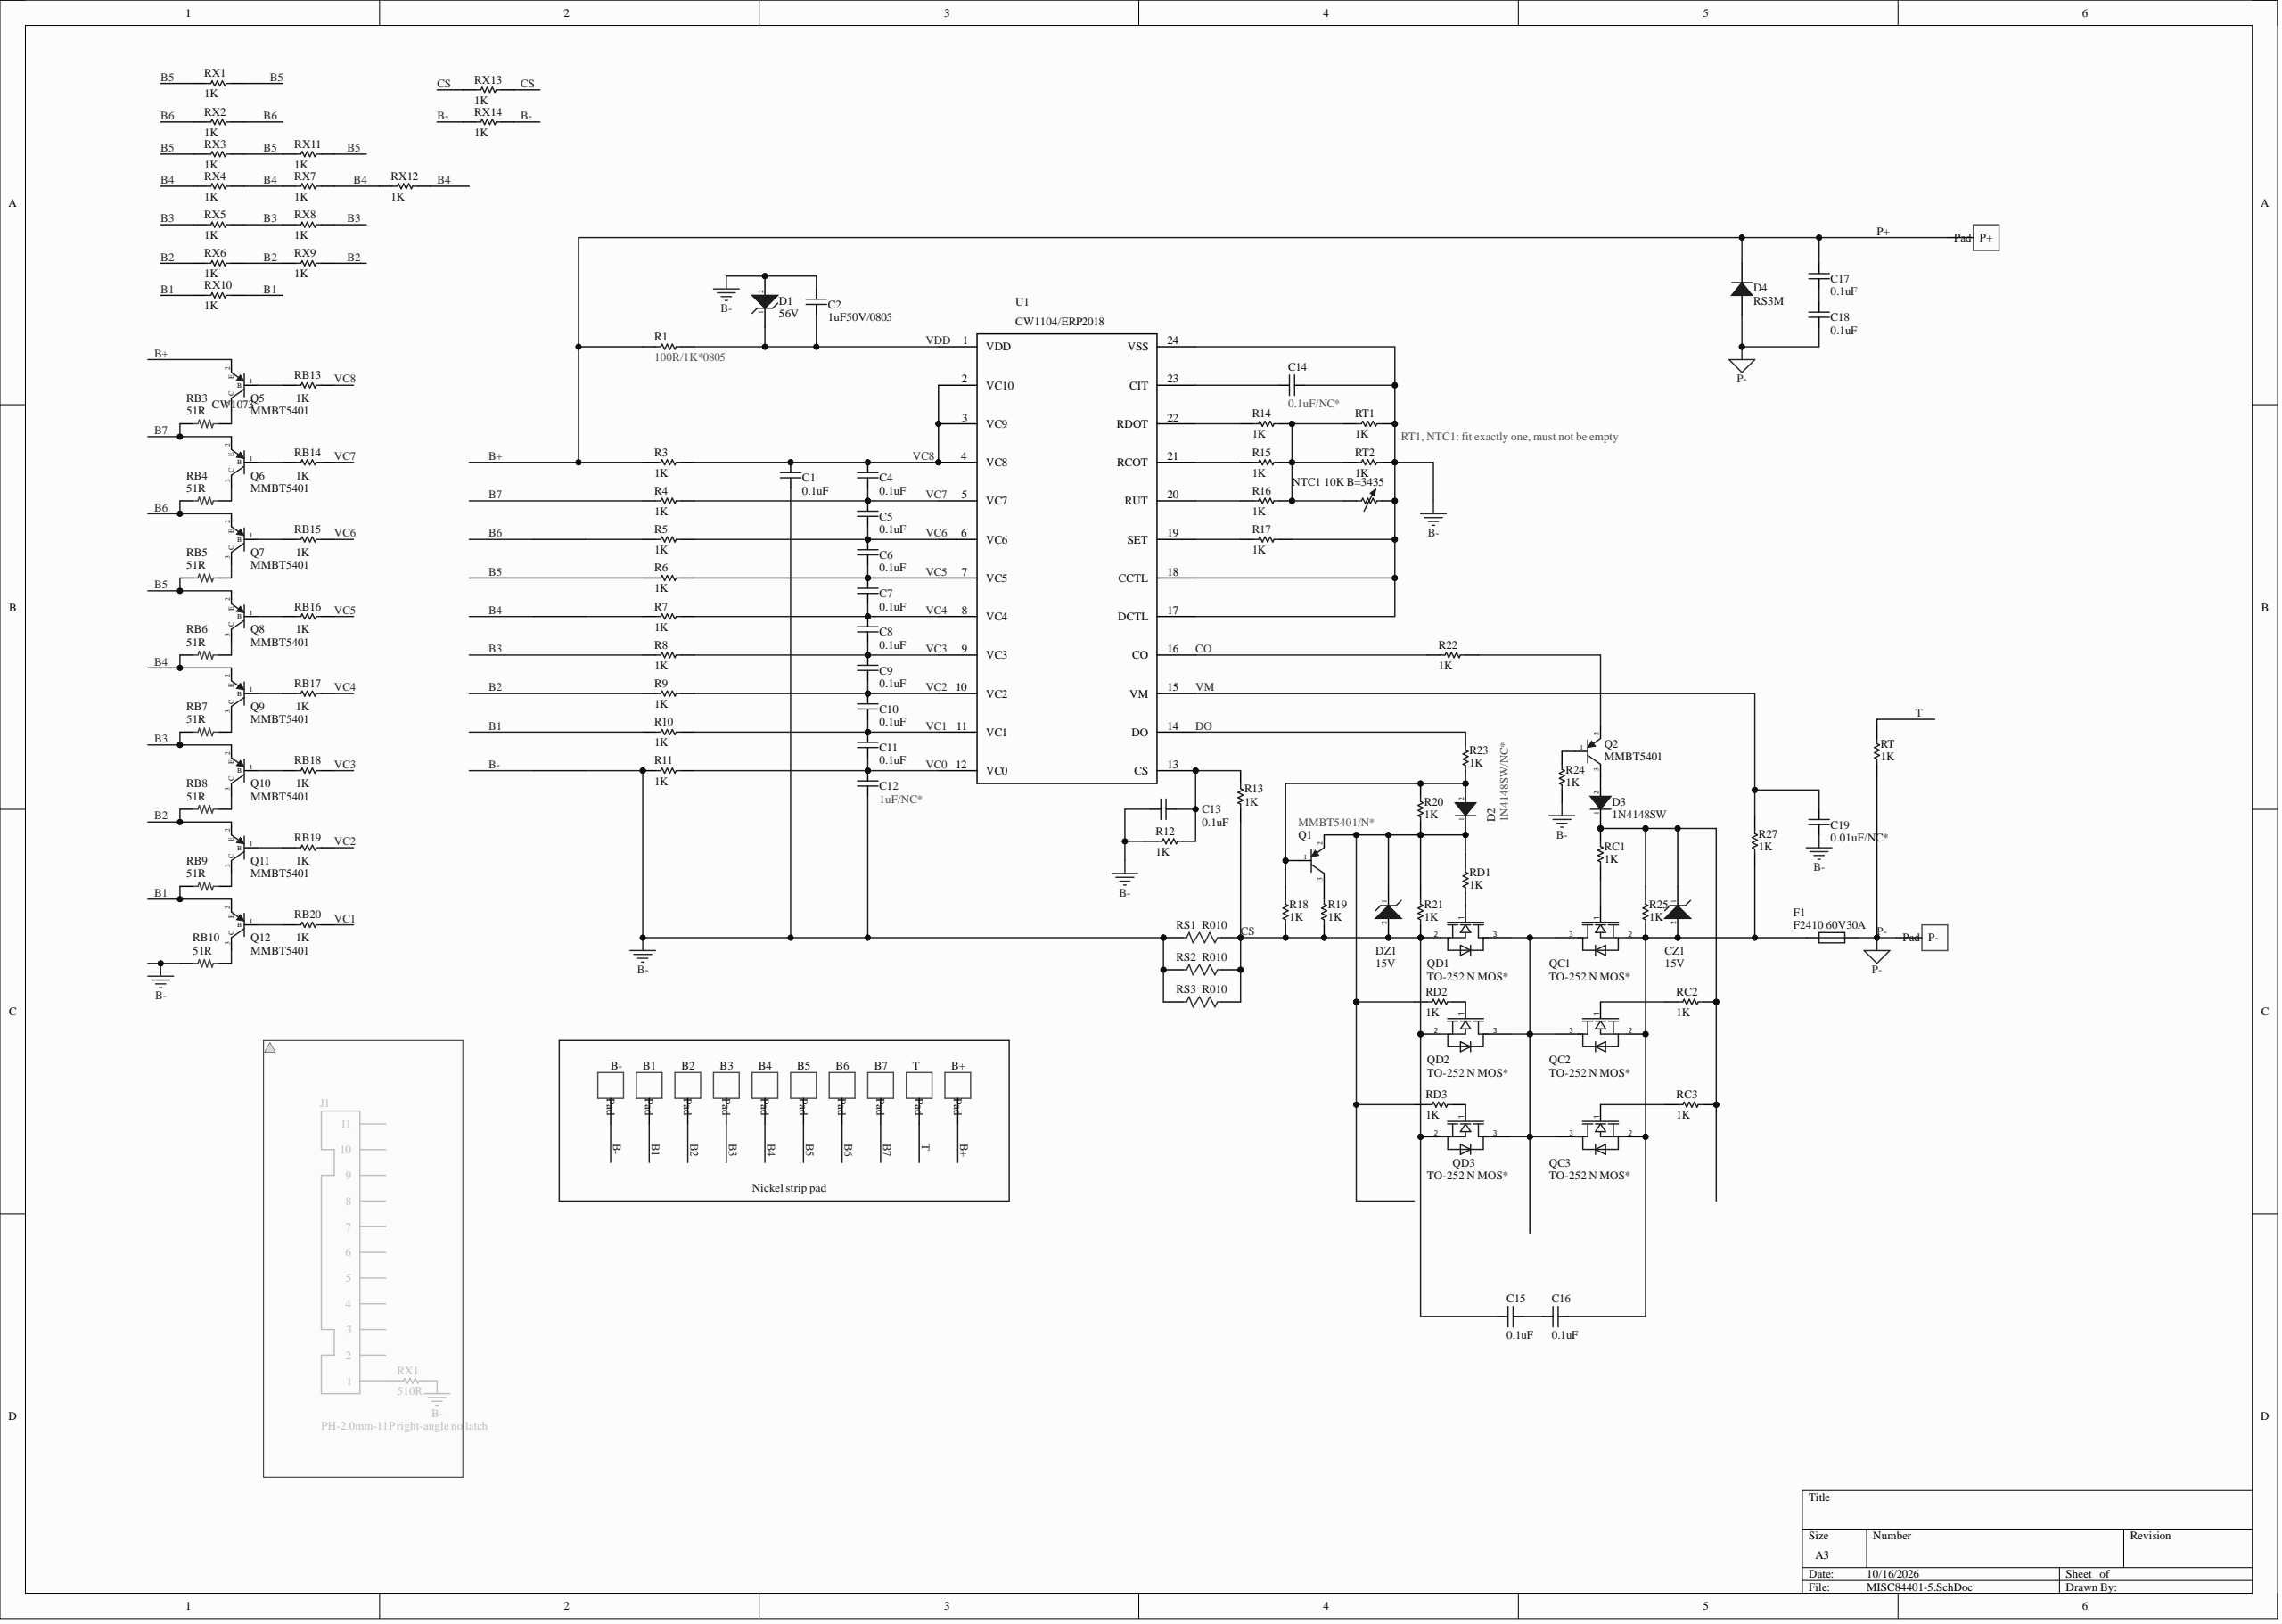Circuit board | Altium Designer | 122 parts | 65 nets
Bill of materials:
Comment,Description,Designator,Footprint,LibRef,Quantity
"Pad","Connection pad (non-through-hole)","B1, B2, B3, B4, B5, B6, B7, B-, B+, P-, P+, T","Pad10X8mm","Pad","12"
"0.1uF","SMD capacitor","C1, C4, C5, C6, C7, C8, C9, C10, C11, C13, C15, C16, C17, C18","C0603A","CAP","14"
"1uF50V/0805","SMD capacitor","C2","C0805A","CAP","1"
"1uF/NC*","SMD capacitor","C12","C0603A","CAP","1"
"0.1uF/NC*","SMD capacitor","C14","C0603A","CAP","1"
"0.01uF/NC*","SMD capacitor","C19","C0603A","CAP","1"
"15V","SMD Zener diode","CZ1, DZ1","SOD323","5V6","2"
"56V","SMD Zener diode","D1","SOD323","5V6","1"
"1N4148SW/NC*","SMD diode","D2","SOD323","1N4148SW","1"
"1N4148SW","SMD diode","D3","SOD323","1N4148SW","1"
"RS3M","SMD diode","D4","SMB(DO-214AA)","RS3M","1"
"F2410 60V30A","","F1","F2410","FUSE","1"
"10K B=3435","SMD thermistor","NTC1","RT2.3X1.2-2","NTC","1"
"MMBT5401/N*","SMD transistor","Q1","SOT23-3","MMBT5401","1"
"MMBT5401","SMD transistor","Q2, Q5, Q6, Q7, Q8, Q9, Q10, Q11, Q12","SOT23-3","MMBT5401","9"
"TO-252 N MOS*","SMD MOS","QC1, QC2, QC3, QD1, QD2, QD3","TO-252","N MOS*","6"
"100R/1K*0805","SMD resistor","R1","R0805A","RES","1"
"1K","SMD resistor","R3, R4, R5, R6, R7, R8, R9, R10, R11, R12, R13, R14, R15, R16, R17, R18, R19, R20, R21, R22, R23, R24, R25, R27, RB13, RB14, RB15, RB16, RB17, RB18, RB19, RB20, RC1, RC2, RC3, RD1, RD2, RD3, RT, RT1, RT2","R0603A","RES","41"
"51R","Alloy SMD resistor","RB3, RB4, RB5, RB6, RB7, RB8, RB9, RB10","R1206A","RES3","8"
"R010","SMD alloy resistor","RS1, RS2, RS3","R2512L","RES2","3"
"1K","SMD resistor","RX1, RX2, RX3, RX4, RX5, RX6, RX7, RX8, RX9, RX10, RX11, RX12","R1206A","RES","12"
"1K","SMD resistor","RX13, RX14","R0805A","RES","2"
"CW1104/ERP2018","Cellwise 7-10S battery protection IC","U1","TSSOP-24(pin间距0.635mm)","CW1104*","1"
Netlist (Protel format):
[
B1
Pad10X8mm
Pad



]
[
B2
Pad10X8mm
Pad



]
[
B3
Pad10X8mm
Pad



]
[
B4
Pad10X8mm
Pad



]
[
B5
Pad10X8mm
Pad



]
[
B6
Pad10X8mm
Pad



]
[
B7
Pad10X8mm
Pad



]
[
B+
Pad10X8mm
Pad



]
[
B-
Pad10X8mm
Pad



]
[
C1
C0603A
0.1uF



]
[
C2
C0805A
1uF50V/0805



]
[
C4
C0603A
0.1uF



]
[
C5
C0603A
0.1uF



]
[
C6
C0603A
0.1uF



]
[
C7
C0603A
0.1uF



]
[
C8
C0603A
0.1uF



]
[
C9
C0603A
0.1uF



]
[
C10
C0603A
0.1uF



]
[
C11
C0603A
0.1uF



]
[
C12
C0603A
1uF/NC*



]
[
C13
C0603A
0.1uF



]
[
C14
C0603A
0.1uF/NC*



]
[
C15
C0603A
0.1uF



]
[
C16
C0603A
0.1uF



]
[
C17
C0603A
0.1uF



]
[
C18
C0603A
0.1uF



]
[
C19
C0603A
0.01uF/NC*



]
[
CZ1
SOD323
15V



]
[
D1
SOD323
56V



]
[
D2
SOD323
1N4148SW/NC*



]
[
D3
SOD323
1N4148SW



]
[
D4
SMB(DO-214AA)
RS3M



]
[
DZ1
SOD323
15V



]
[
F1
F2410
F2410 60V30A



]
[
NTC1
RT2.3X1.2-2
10K B=3435



]
[
P+
Pad10X8mm
Pad



]
[
P-
Pad10X8mm
Pad



]
[
Q1
SOT23-3
MMBT5401/N*



]
[
Q2
SOT23-3
MMBT5401



]
[
Q5
SOT23-3
MMBT5401



]
[
Q6
SOT23-3
MMBT5401



]
[
Q7
SOT23-3
MMBT5401



]
[
Q8
SOT23-3
MMBT5401



]
[
Q9
SOT23-3
MMBT5401



]
[
Q10
SOT23-3
MMBT5401



]
[
Q11
SOT23-3
MMBT5401



]
[
Q12
SOT23-3
MMBT5401



]
[
QC1
TO-252
TO-252 N MOS*



]
[
QC2
TO-252
TO-252 N MOS*



]
[
QC3
TO-252
TO-252 N MOS*



]
[
QD1
TO-252
TO-252 N MOS*



]
[
QD2
TO-252
TO-252 N MOS*



]
[
QD3
TO-252
TO-252 N MOS*



]
[
R1
R0805A
100R/1K*0805



]
[
R3
R0603A
1K



]
[
R4
R0603A
1K



]
[
R5
R0603A
1K



]
[
R6
R0603A
1K



]
[
R7
R0603A
1K



]
[
R8
R0603A
1K



]
[
R9
R0603A
1K



]
[
R10
R0603A
1K



]
[
R11
R0603A
1K



]
[
R12
R0603A
1K



]
[
R13
R0603A
1K



]
[
R14
R0603A
1K



]
[
R15
R0603A
1K



]
[
R16
R0603A
1K



]
[
R17
R0603A
1K



]
[
R18
R0603A
1K



]
[
R19
R0603A
1K



]
[
R20
R0603A
1K



]
[
R21
R0603A
1K



]
[
R22
R0603A
1K



]
[
R23
R0603A
1K



]
[
R24
R0603A
1K



]
[
R25
R0603A
1K



]
[
R27
R0603A
1K



]
[
RB3
R1206A
51R



]
[
RB4
R1206A
51R



]
[
RB5
R1206A
51R



]
[
RB6
R1206A
51R



]
[
RB7
R1206A
51R



]
[
RB8
R1206A
51R



]
[
RB9
R1206A
51R



]
[
RB10
R1206A
51R



]
[
RB13
R0603A
1K



]
[
RB14
R0603A
1K



]
[
RB15
R0603A
1K



]
[
RB16
R0603A
1K



]
[
RB17
R0603A
1K



]
[
RB18
R0603A
1K



]
[
RB19
R0603A
1K



]
[
RB20
R0603A
1K



]
[
RC1
R0603A
1K



]
[
RC2
R0603A
1K



]
[
RC3
R0603A
1K



]
[
RD1
R0603A
1K



]
[
RD2
R0603A
1K



]
[
RD3
R0603A
1K



]
[
RS1
R2512L
R010



]
[
RS2
R2512L
R010



]
[
RS3
R2512L
R010



]
[
RT
R0603A
1K



]
[
RT1
R0603A
1K



]
[
RT2
R0603A
1K



]
[
RX1
R1206A
1K



]
[
RX2
R1206A
1K



]
[
RX3
R1206A
1K



]
[
RX4
R1206A
1K



]
[
RX5
R1206A
1K



]
[
RX6
R1206A
1K



]
[
RX7
R1206A
1K



]
[
RX8
R1206A
1K



]
[
RX9
R1206A
1K



]
[
RX10
R1206A
1K



]
[
RX11
R1206A
1K



]
[
RX12
R1206A
1K



]
[
RX13
R0805A
1K



]
[
RX14
R0805A
1K



]
[
T
Pad10X8mm
Pad



]
[
U1
TSSOP-24(pin间距0.635mm)
CW1104/ERP2018



]
(
VM
C19-1
R27-2
U1-15
)
(
VDD
C2-2
D1-1
R1-2
U1-1
)
(
VC8
C1-2
C4-2
R3-2
RB13-2
U1-2
U1-3
U1-4
)
(
VC7
C4-1
C5-2
R4-2
RB14-2
U1-5
)
(
VC6
C5-1
C6-2
R5-2
RB15-2
U1-6
)
(
VC5
C6-1
C7-2
R6-2
RB16-2
U1-7
)
(
VC4
C7-1
C8-2
R7-2
RB17-2
U1-8
)
(
VC3
C8-1
C9-2
R8-2
RB18-2
U1-9
)
(
VC2
C9-1
C10-2
R9-2
RB19-2
U1-10
)
(
VC1
C10-1
C11-2
R10-2
RB20-2
U1-11
)
(
VC0
C11-1
C12-2
R11-2
U1-12
)
(
T
RT-2
T-1
)
(
P-
C18-1
D4-2
F1-2
P--1
RT-1
)
(
NetR17_1
R17-1
U1-19
)
(
NetR16_1
R16-1
U1-20
)
(
NetR15_1
R15-1
U1-21
)
(
NetR14_1
R14-1
U1-22
)
(
NetQD3_1
QD3-1
RD3-1
)
(
NetQD2_1
QD2-1
RD2-1
)
(
NetQD1_1
QD1-1
RD1-1
)
(
NetQC3_1
QC3-1
RC3-2
)
(
NetQC2_1
QC2-1
RC2-2
)
(
NetQC1_3
QC1-3
QC2-3
QC3-3
QD1-3
QD2-3
QD3-3
)
(
NetQC1_1
QC1-1
RC1-1
)
(
NetQ12_3
Q12-3
RB10-2
)
(
NetQ12_1
Q12-1
RB20-1
)
(
NetQ11_3
Q11-3
RB9-2
)
(
NetQ11_1
Q11-1
RB19-1
)
(
NetQ10_3
Q10-3
RB8-2
)
(
NetQ10_1
Q10-1
RB18-1
)
(
NetQ9_3
Q9-3
RB7-2
)
(
NetQ9_1
Q9-1
RB17-1
)
(
NetQ8_3
Q8-3
RB6-2
)
(
NetQ8_1
Q8-1
RB16-1
)
(
NetQ7_3
Q7-3
RB5-2
)
(
NetQ7_1
Q7-1
RB15-1
)
(
NetQ6_3
Q6-3
RB4-2
)
(
NetQ6_1
Q6-1
RB14-1
)
(
NetQ5_3
Q5-3
RB3-2
)
(
NetQ5_1
Q5-1
RB13-1
)
(
NetQ2_2
Q2-2
R22-2
)
(
NetQ2_1
Q2-1
R24-1
)
(
NetQ1_3
Q1-3
R19-1
)
(
NetNTC1_1
NTC1-1
R14-2
R15-2
R16-2
RT1-1
RT2-1
)
(
NetD3_2
D3-2
Q2-3
)
(
NetD2_2
D2-2
Q1-1
R18-1
R20-1
R23-2
)
(
NetD2_1
D2-1
DZ1-1
Q1-2
R20-2
R21-1
RD1-2
RD2-2
RD3-2
)
(
NetCZ1_1
CZ1-1
D3-1
R25-1
RC1-2
RC2-1
RC3-1
)
(
NetC17_1
C17-1
C18-2
)
(
NetC16_1
C16-1
CZ1-2
F1-1
QC1-2
QC2-2
QC3-2
R25-2
R27-1
)
(
NetC15_1
C15-1
C16-2
)
(
NetC14_2
C14-2
U1-23
)
(
NetC13_2
C13-2
R12-2
R13-1
U1-13
)
(
DO
R23-1
U1-14
)
(
CS
C15-2
DZ1-2
QD1-2
QD2-2
QD3-2
R13-2
R18-2
R19-2
R21-2
RS1-2
RS2-2
RS3-2
RX13-1
RX13-2
)
(
CO
R22-1
U1-16
)
(
B-
B--1
C1-1
C2-1
C12-1
C13-1
C14-1
C19-2
D1-2
NTC1-2
R11-1
R12-1
R17-2
R24-2
RB10-1
RS1-1
RS2-1
RS3-1
RT1-2
RT2-2
RX14-1
RX14-2
U1-17
U1-18
U1-24
)
(
B+
B+-1
C17-2
D4-1
P+-1
Q5-2
R1-1
R3-1
)
(
B7
B7-1
Q6-2
R4-1
RB3-1
)
(
B6
B6-1
Q7-2
R5-1
RB4-1
RX2-1
RX2-2
)
(
B5
B5-1
Q8-2
R6-1
RB5-1
RX1-1
RX1-2
RX3-1
RX3-2
RX11-1
RX11-2
)
(
B4
B4-1
Q9-2
R7-1
RB6-1
RX4-1
RX4-2
RX7-1
RX7-2
RX12-1
RX12-2
)
(
B3
B3-1
Q10-2
R8-1
RB7-1
RX5-1
RX5-2
RX8-1
RX8-2
)
(
B2
B2-1
Q11-2
R9-1
RB8-1
RX6-1
RX6-2
RX9-1
RX9-2
)
(
B1
B1-1
Q12-2
R10-1
RB9-1
RX10-1
RX10-2
)